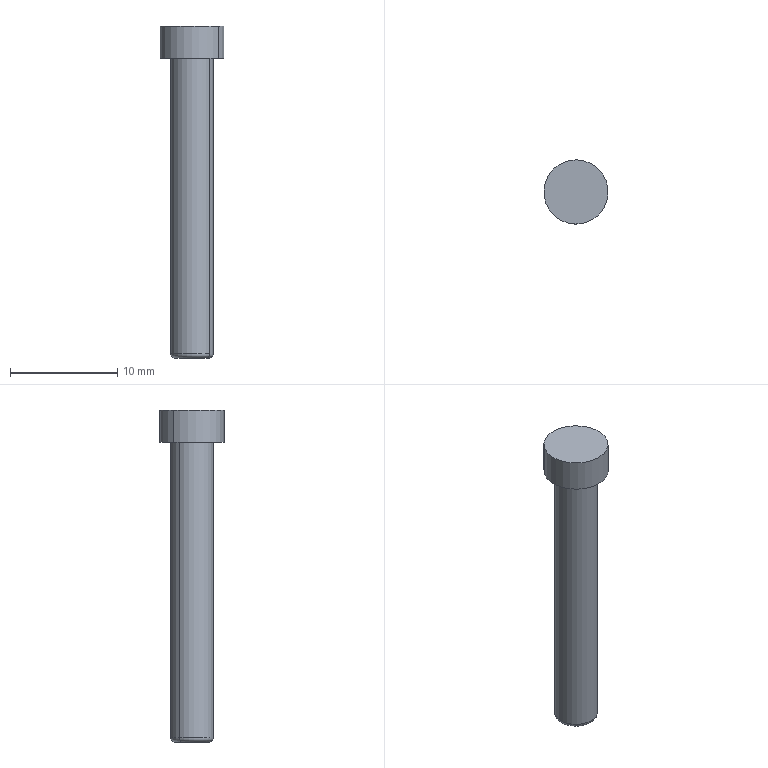Part | SolidWorks | features BaseBody 1 | 1 solid | 9 faces | box 6 x 6 x 31 mm | volume 436.445 mm3 | cylinder 4 | plane 3 | torus 2 | commonest cylinder face diameters 4.001 x2 6 x2
STEP:
#1=CARTESIAN_POINT('',(-72.071,-10.338,50.6));
#2=VERTEX_POINT('',#1);
#3=CARTESIAN_POINT('',(-76.986,-6.896,50.6));
#4=VERTEX_POINT('',#3);
#5=CARTESIAN_POINT('',(-74.528,-8.617,50.6));
#6=DIRECTION('',(0.,0.,1.));
#7=DIRECTION('',(0.8192,-0.5736,0.));
#8=AXIS2_PLACEMENT_3D('',#5,#6,#7);
#9=CIRCLE('',#8,3.);
#10=EDGE_CURVE('',#2,#4,#9,.T.);
#11=ORIENTED_EDGE('',*,*,#10,.T.);
#12=CARTESIAN_POINT('',(-76.986,-6.896,53.6));
#13=VERTEX_POINT('',#12);
#14=CARTESIAN_POINT('',(-76.986,-6.896,50.6));
#15=DIRECTION('',(0.,0.,1.));
#16=VECTOR('',#15,1000.);
#17=LINE('',#14,#16);
#18=EDGE_CURVE('',#4,#13,#17,.T.);
#19=ORIENTED_EDGE('',*,*,#18,.T.);
#20=CARTESIAN_POINT('',(-72.071,-10.338,53.6));
#21=VERTEX_POINT('',#20);
#22=CARTESIAN_POINT('',(-74.528,-8.617,53.6));
#23=DIRECTION('',(0.,0.,-1.));
#24=DIRECTION('',(0.8192,-0.5736,0.));
#25=AXIS2_PLACEMENT_3D('',#22,#23,#24);
#26=CIRCLE('',#25,3.);
#27=EDGE_CURVE('',#13,#21,#26,.T.);
#28=ORIENTED_EDGE('',*,*,#27,.T.);
#29=CARTESIAN_POINT('',(-72.071,-10.338,50.6));
#30=DIRECTION('',(0.,0.,1.));
#31=VECTOR('',#30,1000.);
#32=LINE('',#29,#31);
#33=EDGE_CURVE('',#2,#21,#32,.T.);
#34=ORIENTED_EDGE('',*,*,#33,.F.);
#35=EDGE_LOOP('',(#11,#19,#28,#34));
#36=FACE_OUTER_BOUND('',#35,.T.);
#37=CARTESIAN_POINT('',(-74.528,-8.617,50.6));
#38=DIRECTION('',(0.,0.,1.));
#39=DIRECTION('',(0.8192,-0.5736,0.));
#40=AXIS2_PLACEMENT_3D('',#37,#38,#39);
#41=CYLINDRICAL_SURFACE('',#40,3.);
#42=ADVANCED_FACE('',(#36),#41,.T.);
#43=CARTESIAN_POINT('',(-72.89,-9.764,23.));
#44=VERTEX_POINT('',#43);
#45=CARTESIAN_POINT('',(-76.167,-7.47,23.));
#46=VERTEX_POINT('',#45);
#47=CARTESIAN_POINT('',(-74.528,-8.617,23.));
#48=DIRECTION('',(0.,0.,1.));
#49=DIRECTION('',(-0.8192,0.5736,0.));
#50=AXIS2_PLACEMENT_3D('',#47,#48,#49);
#51=CIRCLE('',#50,2.);
#52=EDGE_CURVE('',#44,#46,#51,.T.);
#53=ORIENTED_EDGE('',*,*,#52,.F.);
#54=CARTESIAN_POINT('',(-73.218,-9.535,22.6));
#55=VERTEX_POINT('',#54);
#56=CARTESIAN_POINT('',(-73.218,-9.535,23.));
#57=DIRECTION('',(0.5736,0.8192,0.));
#58=DIRECTION('',(-0.8192,0.5736,0.));
#59=AXIS2_PLACEMENT_3D('',#56,#57,#58);
#60=CIRCLE('',#59,0.4001);
#61=EDGE_CURVE('',#44,#55,#60,.T.);
#62=ORIENTED_EDGE('',*,*,#61,.T.);
#63=CARTESIAN_POINT('',(-75.839,-7.699,22.6));
#64=VERTEX_POINT('',#63);
#65=CARTESIAN_POINT('',(-74.528,-8.617,22.6));
#66=DIRECTION('',(0.,0.,-1.));
#67=DIRECTION('',(-0.8192,0.5736,0.));
#68=AXIS2_PLACEMENT_3D('',#65,#66,#67);
#69=CIRCLE('',#68,1.6);
#70=EDGE_CURVE('',#64,#55,#69,.T.);
#71=ORIENTED_EDGE('',*,*,#70,.F.);
#72=CARTESIAN_POINT('',(-75.839,-7.699,23.));
#73=DIRECTION('',(-0.5736,-0.8192,0.));
#74=DIRECTION('',(0.8192,-0.5736,0.));
#75=AXIS2_PLACEMENT_3D('',#72,#73,#74);
#76=CIRCLE('',#75,0.4001);
#77=EDGE_CURVE('',#46,#64,#76,.T.);
#78=ORIENTED_EDGE('',*,*,#77,.F.);
#79=EDGE_LOOP('',(#53,#62,#71,#78));
#80=FACE_OUTER_BOUND('',#79,.T.);
#81=CARTESIAN_POINT('',(-74.528,-8.617,23.));
#82=DIRECTION('',(0.,0.,-1.));
#83=DIRECTION('',(-0.8192,0.5736,0.));
#84=AXIS2_PLACEMENT_3D('',#81,#82,#83);
#85=TOROIDAL_SURFACE('',#84,1.6,0.4001);
#86=ADVANCED_FACE('',(#80),#85,.T.);
#87=ORIENTED_EDGE('',*,*,#52,.T.);
#88=CARTESIAN_POINT('',(-76.167,-7.47,50.6));
#89=VERTEX_POINT('',#88);
#90=CARTESIAN_POINT('',(-76.167,-7.47,22.6));
#91=DIRECTION('',(0.,0.,1.));
#92=VECTOR('',#91,1000.);
#93=LINE('',#90,#92);
#94=EDGE_CURVE('',#46,#89,#93,.T.);
#95=ORIENTED_EDGE('',*,*,#94,.T.);
#96=CARTESIAN_POINT('',(-72.89,-9.764,50.6));
#97=VERTEX_POINT('',#96);
#98=CARTESIAN_POINT('',(-74.528,-8.617,50.6));
#99=DIRECTION('',(0.,0.,-1.));
#100=DIRECTION('',(0.8192,-0.5736,0.));
#101=AXIS2_PLACEMENT_3D('',#98,#99,#100);
#102=CIRCLE('',#101,2.);
#103=EDGE_CURVE('',#89,#97,#102,.T.);
#104=ORIENTED_EDGE('',*,*,#103,.T.);
#105=CARTESIAN_POINT('',(-72.89,-9.764,22.6));
#106=DIRECTION('',(0.,0.,1.));
#107=VECTOR('',#106,1000.);
#108=LINE('',#105,#107);
#109=EDGE_CURVE('',#44,#97,#108,.T.);
#110=ORIENTED_EDGE('',*,*,#109,.F.);
#111=EDGE_LOOP('',(#87,#95,#104,#110));
#112=FACE_OUTER_BOUND('',#111,.T.);
#113=CARTESIAN_POINT('',(-74.528,-8.617,22.6));
#114=DIRECTION('',(0.,0.,1.));
#115=DIRECTION('',(0.8192,-0.5736,0.));
#116=AXIS2_PLACEMENT_3D('',#113,#114,#115);
#117=CYLINDRICAL_SURFACE('',#116,2.);
#118=ADVANCED_FACE('',(#112),#117,.T.);
#119=ORIENTED_EDGE('',*,*,#70,.T.);
#120=CARTESIAN_POINT('',(-74.528,-8.617,22.6));
#121=DIRECTION('',(0.,0.,-1.));
#122=DIRECTION('',(-0.8192,0.5736,0.));
#123=AXIS2_PLACEMENT_3D('',#120,#121,#122);
#124=CIRCLE('',#123,1.6);
#125=EDGE_CURVE('',#55,#64,#124,.T.);
#126=ORIENTED_EDGE('',*,*,#125,.T.);
#127=EDGE_LOOP('',(#119,#126));
#128=FACE_OUTER_BOUND('',#127,.T.);
#129=CARTESIAN_POINT('',(-74.528,-8.617,22.6));
#130=DIRECTION('',(0.,0.,-1.));
#131=DIRECTION('',(-0.8192,0.5736,0.));
#132=AXIS2_PLACEMENT_3D('',#129,#130,#131);
#133=PLANE('',#132);
#134=ADVANCED_FACE('',(#128),#133,.T.);
#135=ORIENTED_EDGE('',*,*,#94,.F.);
#136=CARTESIAN_POINT('',(-74.528,-8.617,23.));
#137=DIRECTION('',(0.,0.,1.));
#138=DIRECTION('',(-0.8192,0.5736,0.));
#139=AXIS2_PLACEMENT_3D('',#136,#137,#138);
#140=CIRCLE('',#139,2.);
#141=EDGE_CURVE('',#46,#44,#140,.T.);
#142=ORIENTED_EDGE('',*,*,#141,.T.);
#143=ORIENTED_EDGE('',*,*,#109,.T.);
#144=CARTESIAN_POINT('',(-74.528,-8.617,50.6));
#145=DIRECTION('',(0.,0.,-1.));
#146=DIRECTION('',(0.8192,-0.5736,0.));
#147=AXIS2_PLACEMENT_3D('',#144,#145,#146);
#148=CIRCLE('',#147,2.);
#149=EDGE_CURVE('',#97,#89,#148,.T.);
#150=ORIENTED_EDGE('',*,*,#149,.T.);
#151=EDGE_LOOP('',(#135,#142,#143,#150));
#152=FACE_OUTER_BOUND('',#151,.T.);
#153=CARTESIAN_POINT('',(-74.528,-8.617,22.6));
#154=DIRECTION('',(0.,0.,1.));
#155=DIRECTION('',(0.8192,-0.5736,0.));
#156=AXIS2_PLACEMENT_3D('',#153,#154,#155);
#157=CYLINDRICAL_SURFACE('',#156,2.);
#158=ADVANCED_FACE('',(#152),#157,.T.);
#159=ORIENTED_EDGE('',*,*,#61,.F.);
#160=ORIENTED_EDGE('',*,*,#141,.F.);
#161=ORIENTED_EDGE('',*,*,#77,.T.);
#162=ORIENTED_EDGE('',*,*,#125,.F.);
#163=EDGE_LOOP('',(#159,#160,#161,#162));
#164=FACE_OUTER_BOUND('',#163,.T.);
#165=CARTESIAN_POINT('',(-74.528,-8.617,23.));
#166=DIRECTION('',(0.,0.,-1.));
#167=DIRECTION('',(-0.8192,0.5736,0.));
#168=AXIS2_PLACEMENT_3D('',#165,#166,#167);
#169=TOROIDAL_SURFACE('',#168,1.6,0.4001);
#170=ADVANCED_FACE('',(#164),#169,.T.);
#171=CARTESIAN_POINT('',(-74.528,-8.617,53.6));
#172=DIRECTION('',(0.,0.,-1.));
#173=DIRECTION('',(0.8192,-0.5736,0.));
#174=AXIS2_PLACEMENT_3D('',#171,#172,#173);
#175=CIRCLE('',#174,3.);
#176=EDGE_CURVE('',#21,#13,#175,.T.);
#177=ORIENTED_EDGE('',*,*,#176,.F.);
#178=ORIENTED_EDGE('',*,*,#27,.F.);
#179=EDGE_LOOP('',(#177,#178));
#180=FACE_OUTER_BOUND('',#179,.T.);
#181=CARTESIAN_POINT('',(-74.528,-8.617,53.6));
#182=DIRECTION('',(0.,0.,1.));
#183=DIRECTION('',(0.8192,-0.5736,0.));
#184=AXIS2_PLACEMENT_3D('',#181,#182,#183);
#185=PLANE('',#184);
#186=ADVANCED_FACE('',(#180),#185,.T.);
#187=ORIENTED_EDGE('',*,*,#149,.F.);
#188=ORIENTED_EDGE('',*,*,#103,.F.);
#189=EDGE_LOOP('',(#187,#188));
#190=FACE_BOUND('',#189,.T.);
#191=ORIENTED_EDGE('',*,*,#10,.F.);
#192=CARTESIAN_POINT('',(-74.528,-8.617,50.6));
#193=DIRECTION('',(0.,0.,1.));
#194=DIRECTION('',(0.8192,-0.5736,0.));
#195=AXIS2_PLACEMENT_3D('',#192,#193,#194);
#196=CIRCLE('',#195,3.);
#197=EDGE_CURVE('',#4,#2,#196,.T.);
#198=ORIENTED_EDGE('',*,*,#197,.F.);
#199=EDGE_LOOP('',(#191,#198));
#200=FACE_OUTER_BOUND('',#199,.T.);
#201=CARTESIAN_POINT('',(-74.528,-8.617,50.6));
#202=DIRECTION('',(0.,0.,-1.));
#203=DIRECTION('',(-0.8192,0.5736,0.));
#204=AXIS2_PLACEMENT_3D('',#201,#202,#203);
#205=PLANE('',#204);
#206=ADVANCED_FACE('',(#190,#200),#205,.T.);
#207=ORIENTED_EDGE('',*,*,#18,.F.);
#208=ORIENTED_EDGE('',*,*,#197,.T.);
#209=ORIENTED_EDGE('',*,*,#33,.T.);
#210=ORIENTED_EDGE('',*,*,#176,.T.);
#211=EDGE_LOOP('',(#207,#208,#209,#210));
#212=FACE_OUTER_BOUND('',#211,.T.);
#213=CARTESIAN_POINT('',(-74.528,-8.617,50.6));
#214=DIRECTION('',(0.,0.,1.));
#215=DIRECTION('',(0.8192,-0.5736,0.));
#216=AXIS2_PLACEMENT_3D('',#213,#214,#215);
#217=CYLINDRICAL_SURFACE('',#216,3.);
#218=ADVANCED_FACE('',(#212),#217,.T.);
#219=CLOSED_SHELL('',(#42,#86,#118,#134,#158,#170,#186,#206,#218));
#220=MANIFOLD_SOLID_BREP('',#219);
#221=CARTESIAN_POINT('',(0.,0.,0.));
#222=DIRECTION('',(0.,0.,1.));
#223=DIRECTION('',(1.,0.,0.));
#224=AXIS2_PLACEMENT_3D('',#221,#222,#223);
#225=(LENGTH_UNIT()NAMED_UNIT(*)SI_UNIT(.MILLI.,.METRE.));
#226=UNCERTAINTY_MEASURE_WITH_UNIT(LENGTH_MEASURE(0.00001),#225,'','');
#227=(NAMED_UNIT(*)PLANE_ANGLE_UNIT()SI_UNIT($,.RADIAN.));
#228=(NAMED_UNIT(*)SI_UNIT($,.STERADIAN.)SOLID_ANGLE_UNIT());
#229=(GEOMETRIC_REPRESENTATION_CONTEXT(3)GLOBAL_UNCERTAINTY_ASSIGNED_CONTEXT((#226))GLOBAL_UNIT_ASSIGNED_CONTEXT((#225,#227,#228))REPRESENTATION_CONTEXT('',''));
#230=ADVANCED_BREP_SHAPE_REPRESENTATION('',(#220,#224),#229);